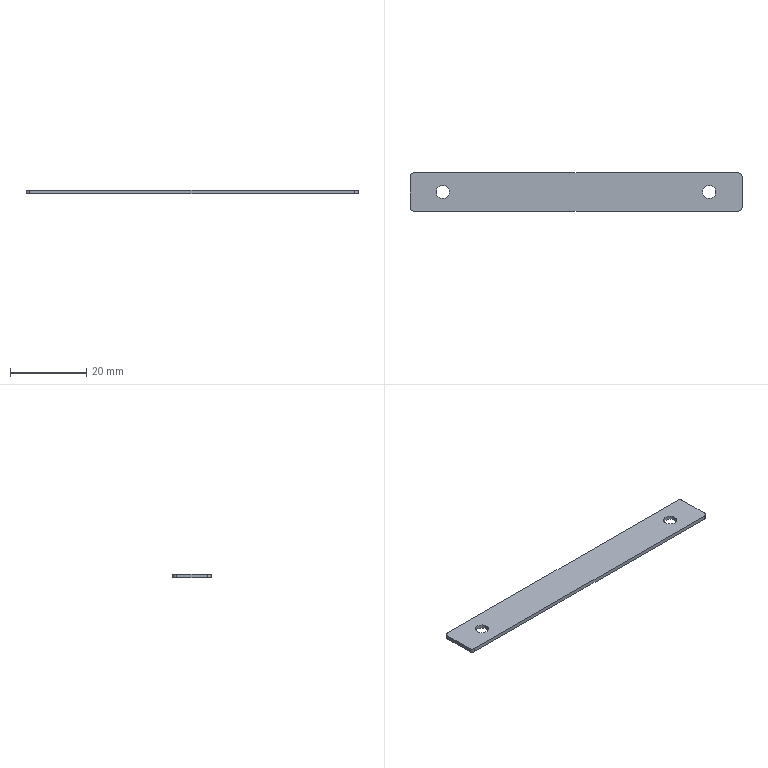Part | STEP file | LES120 steel strip pressure plate^FTH120-PD-direct-drive motor | 1 solid | 14 faces | box 87 x 10 x 1 mm | volume 849.899 mm3 | cylinder 8 | plane 6 | commonest cylinder face diameters 2 x4 3.5 x4
STEP:
#1=CARTESIAN_POINT('',(-36.65,0.,0.));
#2=VERTEX_POINT('',#1);
#3=CARTESIAN_POINT('',(-33.15,0.,0.));
#4=VERTEX_POINT('',#3);
#5=CARTESIAN_POINT('',(-34.9,0.,0.));
#6=DIRECTION('',(0.,0.,1.));
#7=DIRECTION('',(1.,0.,0.));
#8=AXIS2_PLACEMENT_3D('',#5,#6,#7);
#9=CIRCLE('',#8,1.75);
#10=EDGE_CURVE('',#2,#4,#9,.T.);
#11=ORIENTED_EDGE('',*,*,#10,.F.);
#12=CARTESIAN_POINT('',(-36.65,0.,1.));
#13=VERTEX_POINT('',#12);
#14=CARTESIAN_POINT('',(-36.65,0.,0.));
#15=DIRECTION('',(0.,0.,1.));
#16=VECTOR('',#15,1000.);
#17=LINE('',#14,#16);
#18=EDGE_CURVE('',#2,#13,#17,.T.);
#19=ORIENTED_EDGE('',*,*,#18,.T.);
#20=CARTESIAN_POINT('',(-33.15,0.,1.));
#21=VERTEX_POINT('',#20);
#22=CARTESIAN_POINT('',(-34.9,0.,1.));
#23=DIRECTION('',(0.,0.,1.));
#24=DIRECTION('',(1.,0.,0.));
#25=AXIS2_PLACEMENT_3D('',#22,#23,#24);
#26=CIRCLE('',#25,1.75);
#27=EDGE_CURVE('',#13,#21,#26,.T.);
#28=ORIENTED_EDGE('',*,*,#27,.T.);
#29=CARTESIAN_POINT('',(-33.15,0.,0.));
#30=DIRECTION('',(0.,0.,1.));
#31=VECTOR('',#30,1000.);
#32=LINE('',#29,#31);
#33=EDGE_CURVE('',#4,#21,#32,.T.);
#34=ORIENTED_EDGE('',*,*,#33,.F.);
#35=EDGE_LOOP('',(#11,#19,#28,#34));
#36=FACE_OUTER_BOUND('',#35,.T.);
#37=CARTESIAN_POINT('',(-34.9,0.,0.));
#38=DIRECTION('',(0.,0.,1.));
#39=DIRECTION('',(1.,0.,0.));
#40=AXIS2_PLACEMENT_3D('',#37,#38,#39);
#41=CYLINDRICAL_SURFACE('',#40,1.75);
#42=ADVANCED_FACE('',(#36),#41,.F.);
#43=CARTESIAN_POINT('',(33.15,0.,0.));
#44=VERTEX_POINT('',#43);
#45=CARTESIAN_POINT('',(36.65,0.,0.));
#46=VERTEX_POINT('',#45);
#47=CARTESIAN_POINT('',(34.9,0.,0.));
#48=DIRECTION('',(0.,0.,1.));
#49=DIRECTION('',(1.,0.,0.));
#50=AXIS2_PLACEMENT_3D('',#47,#48,#49);
#51=CIRCLE('',#50,1.75);
#52=EDGE_CURVE('',#44,#46,#51,.T.);
#53=ORIENTED_EDGE('',*,*,#52,.F.);
#54=CARTESIAN_POINT('',(33.15,0.,1.));
#55=VERTEX_POINT('',#54);
#56=CARTESIAN_POINT('',(33.15,0.,0.));
#57=DIRECTION('',(0.,0.,1.));
#58=VECTOR('',#57,1000.);
#59=LINE('',#56,#58);
#60=EDGE_CURVE('',#44,#55,#59,.T.);
#61=ORIENTED_EDGE('',*,*,#60,.T.);
#62=CARTESIAN_POINT('',(36.65,0.,1.));
#63=VERTEX_POINT('',#62);
#64=CARTESIAN_POINT('',(34.9,0.,1.));
#65=DIRECTION('',(0.,0.,1.));
#66=DIRECTION('',(1.,0.,0.));
#67=AXIS2_PLACEMENT_3D('',#64,#65,#66);
#68=CIRCLE('',#67,1.75);
#69=EDGE_CURVE('',#55,#63,#68,.T.);
#70=ORIENTED_EDGE('',*,*,#69,.T.);
#71=CARTESIAN_POINT('',(36.65,0.,0.));
#72=DIRECTION('',(0.,0.,1.));
#73=VECTOR('',#72,1000.);
#74=LINE('',#71,#73);
#75=EDGE_CURVE('',#46,#63,#74,.T.);
#76=ORIENTED_EDGE('',*,*,#75,.F.);
#77=EDGE_LOOP('',(#53,#61,#70,#76));
#78=FACE_OUTER_BOUND('',#77,.T.);
#79=CARTESIAN_POINT('',(34.9,0.,0.));
#80=DIRECTION('',(0.,0.,1.));
#81=DIRECTION('',(1.,0.,0.));
#82=AXIS2_PLACEMENT_3D('',#79,#80,#81);
#83=CYLINDRICAL_SURFACE('',#82,1.75);
#84=ADVANCED_FACE('',(#78),#83,.F.);
#85=CARTESIAN_POINT('',(42.5,5.,1.));
#86=VERTEX_POINT('',#85);
#87=CARTESIAN_POINT('',(43.5,4.,1.));
#88=VERTEX_POINT('',#87);
#89=CARTESIAN_POINT('',(42.5,4.,1.));
#90=DIRECTION('',(0.,0.,-1.));
#91=DIRECTION('',(-1.,0.,0.));
#92=AXIS2_PLACEMENT_3D('',#89,#90,#91);
#93=CIRCLE('',#92,1.);
#94=EDGE_CURVE('',#86,#88,#93,.T.);
#95=ORIENTED_EDGE('',*,*,#94,.F.);
#96=CARTESIAN_POINT('',(-42.5,5.,1.));
#97=VERTEX_POINT('',#96);
#98=CARTESIAN_POINT('',(0.,5.,1.));
#99=DIRECTION('',(1.,0.,0.));
#100=VECTOR('',#99,1000.);
#101=LINE('',#98,#100);
#102=EDGE_CURVE('',#97,#86,#101,.T.);
#103=ORIENTED_EDGE('',*,*,#102,.F.);
#104=CARTESIAN_POINT('',(-43.5,4.,1.));
#105=VERTEX_POINT('',#104);
#106=CARTESIAN_POINT('',(-42.5,4.,1.));
#107=DIRECTION('',(0.,0.,-1.));
#108=DIRECTION('',(-1.,0.,0.));
#109=AXIS2_PLACEMENT_3D('',#106,#107,#108);
#110=CIRCLE('',#109,1.);
#111=EDGE_CURVE('',#105,#97,#110,.T.);
#112=ORIENTED_EDGE('',*,*,#111,.F.);
#113=CARTESIAN_POINT('',(-43.5,-4.,1.));
#114=VERTEX_POINT('',#113);
#115=CARTESIAN_POINT('',(-43.5,0.,1.));
#116=DIRECTION('',(0.,1.,0.));
#117=VECTOR('',#116,1000.);
#118=LINE('',#115,#117);
#119=EDGE_CURVE('',#114,#105,#118,.T.);
#120=ORIENTED_EDGE('',*,*,#119,.F.);
#121=CARTESIAN_POINT('',(-42.5,-5.,1.));
#122=VERTEX_POINT('',#121);
#123=CARTESIAN_POINT('',(-42.5,-4.,1.));
#124=DIRECTION('',(0.,0.,-1.));
#125=DIRECTION('',(-1.,0.,0.));
#126=AXIS2_PLACEMENT_3D('',#123,#124,#125);
#127=CIRCLE('',#126,1.);
#128=EDGE_CURVE('',#122,#114,#127,.T.);
#129=ORIENTED_EDGE('',*,*,#128,.F.);
#130=CARTESIAN_POINT('',(42.5,-5.,1.));
#131=VERTEX_POINT('',#130);
#132=CARTESIAN_POINT('',(0.,-5.,1.));
#133=DIRECTION('',(-1.,0.,0.));
#134=VECTOR('',#133,1000.);
#135=LINE('',#132,#134);
#136=EDGE_CURVE('',#131,#122,#135,.T.);
#137=ORIENTED_EDGE('',*,*,#136,.F.);
#138=CARTESIAN_POINT('',(43.5,-4.,1.));
#139=VERTEX_POINT('',#138);
#140=CARTESIAN_POINT('',(42.5,-4.,1.));
#141=DIRECTION('',(0.,0.,-1.));
#142=DIRECTION('',(-1.,0.,0.));
#143=AXIS2_PLACEMENT_3D('',#140,#141,#142);
#144=CIRCLE('',#143,1.);
#145=EDGE_CURVE('',#139,#131,#144,.T.);
#146=ORIENTED_EDGE('',*,*,#145,.F.);
#147=CARTESIAN_POINT('',(43.5,0.,1.));
#148=DIRECTION('',(0.,-1.,0.));
#149=VECTOR('',#148,1000.);
#150=LINE('',#147,#149);
#151=EDGE_CURVE('',#88,#139,#150,.T.);
#152=ORIENTED_EDGE('',*,*,#151,.F.);
#153=EDGE_LOOP('',(#95,#103,#112,#120,#129,#137,#146,#152));
#154=FACE_OUTER_BOUND('',#153,.T.);
#155=CARTESIAN_POINT('',(-34.9,0.,1.));
#156=DIRECTION('',(0.,0.,1.));
#157=DIRECTION('',(1.,0.,0.));
#158=AXIS2_PLACEMENT_3D('',#155,#156,#157);
#159=CIRCLE('',#158,1.75);
#160=EDGE_CURVE('',#21,#13,#159,.T.);
#161=ORIENTED_EDGE('',*,*,#160,.F.);
#162=ORIENTED_EDGE('',*,*,#27,.F.);
#163=EDGE_LOOP('',(#161,#162));
#164=FACE_BOUND('',#163,.T.);
#165=CARTESIAN_POINT('',(34.9,0.,1.));
#166=DIRECTION('',(0.,0.,1.));
#167=DIRECTION('',(1.,0.,0.));
#168=AXIS2_PLACEMENT_3D('',#165,#166,#167);
#169=CIRCLE('',#168,1.75);
#170=EDGE_CURVE('',#63,#55,#169,.T.);
#171=ORIENTED_EDGE('',*,*,#170,.F.);
#172=ORIENTED_EDGE('',*,*,#69,.F.);
#173=EDGE_LOOP('',(#171,#172));
#174=FACE_BOUND('',#173,.T.);
#175=CARTESIAN_POINT('',(0.,0.,1.));
#176=DIRECTION('',(0.,0.,-1.));
#177=DIRECTION('',(-1.,0.,0.));
#178=AXIS2_PLACEMENT_3D('',#175,#176,#177);
#179=PLANE('',#178);
#180=ADVANCED_FACE('',(#154,#164,#174),#179,.F.);
#181=CARTESIAN_POINT('',(43.5,4.,0.));
#182=VERTEX_POINT('',#181);
#183=CARTESIAN_POINT('',(43.5,4.,1.));
#184=DIRECTION('',(0.,0.,-1.));
#185=VECTOR('',#184,1000.);
#186=LINE('',#183,#185);
#187=EDGE_CURVE('',#88,#182,#186,.T.);
#188=ORIENTED_EDGE('',*,*,#187,.F.);
#189=ORIENTED_EDGE('',*,*,#151,.T.);
#190=CARTESIAN_POINT('',(43.5,-4.,0.));
#191=VERTEX_POINT('',#190);
#192=CARTESIAN_POINT('',(43.5,-4.,1.));
#193=DIRECTION('',(0.,0.,1.));
#194=VECTOR('',#193,1000.);
#195=LINE('',#192,#194);
#196=EDGE_CURVE('',#191,#139,#195,.T.);
#197=ORIENTED_EDGE('',*,*,#196,.F.);
#198=CARTESIAN_POINT('',(43.5,-5.,0.));
#199=DIRECTION('',(0.,-1.,0.));
#200=VECTOR('',#199,1000.);
#201=LINE('',#198,#200);
#202=EDGE_CURVE('',#182,#191,#201,.T.);
#203=ORIENTED_EDGE('',*,*,#202,.F.);
#204=EDGE_LOOP('',(#188,#189,#197,#203));
#205=FACE_OUTER_BOUND('',#204,.T.);
#206=CARTESIAN_POINT('',(43.5,-5.,1.));
#207=DIRECTION('',(-1.,0.,0.));
#208=DIRECTION('',(0.,0.,1.));
#209=AXIS2_PLACEMENT_3D('',#206,#207,#208);
#210=PLANE('',#209);
#211=ADVANCED_FACE('',(#205),#210,.F.);
#212=CARTESIAN_POINT('',(42.5,5.,0.));
#213=VERTEX_POINT('',#212);
#214=CARTESIAN_POINT('',(42.5,4.,0.));
#215=DIRECTION('',(0.,0.,1.));
#216=DIRECTION('',(-1.,0.,0.));
#217=AXIS2_PLACEMENT_3D('',#214,#215,#216);
#218=CIRCLE('',#217,1.);
#219=EDGE_CURVE('',#182,#213,#218,.T.);
#220=ORIENTED_EDGE('',*,*,#219,.T.);
#221=CARTESIAN_POINT('',(42.5,5.,1.));
#222=DIRECTION('',(0.,0.,1.));
#223=VECTOR('',#222,1000.);
#224=LINE('',#221,#223);
#225=EDGE_CURVE('',#213,#86,#224,.T.);
#226=ORIENTED_EDGE('',*,*,#225,.T.);
#227=ORIENTED_EDGE('',*,*,#94,.T.);
#228=ORIENTED_EDGE('',*,*,#187,.T.);
#229=EDGE_LOOP('',(#220,#226,#227,#228));
#230=FACE_OUTER_BOUND('',#229,.T.);
#231=CARTESIAN_POINT('',(42.5,4.,1.));
#232=DIRECTION('',(0.,0.,-1.));
#233=DIRECTION('',(-1.,0.,0.));
#234=AXIS2_PLACEMENT_3D('',#231,#232,#233);
#235=CYLINDRICAL_SURFACE('',#234,1.);
#236=ADVANCED_FACE('',(#230),#235,.T.);
#237=ORIENTED_EDGE('',*,*,#225,.F.);
#238=CARTESIAN_POINT('',(-42.5,5.,0.));
#239=VERTEX_POINT('',#238);
#240=CARTESIAN_POINT('',(-43.5,5.,0.));
#241=DIRECTION('',(1.,0.,0.));
#242=VECTOR('',#241,1000.);
#243=LINE('',#240,#242);
#244=EDGE_CURVE('',#239,#213,#243,.T.);
#245=ORIENTED_EDGE('',*,*,#244,.F.);
#246=CARTESIAN_POINT('',(-42.5,5.,1.));
#247=DIRECTION('',(0.,0.,-1.));
#248=VECTOR('',#247,1000.);
#249=LINE('',#246,#248);
#250=EDGE_CURVE('',#97,#239,#249,.T.);
#251=ORIENTED_EDGE('',*,*,#250,.F.);
#252=ORIENTED_EDGE('',*,*,#102,.T.);
#253=EDGE_LOOP('',(#237,#245,#251,#252));
#254=FACE_OUTER_BOUND('',#253,.T.);
#255=CARTESIAN_POINT('',(-43.5,5.,1.));
#256=DIRECTION('',(0.,-1.,0.));
#257=DIRECTION('',(0.,0.,-1.));
#258=AXIS2_PLACEMENT_3D('',#255,#256,#257);
#259=PLANE('',#258);
#260=ADVANCED_FACE('',(#254),#259,.F.);
#261=CARTESIAN_POINT('',(-43.5,4.,0.));
#262=VERTEX_POINT('',#261);
#263=CARTESIAN_POINT('',(-42.5,4.,0.));
#264=DIRECTION('',(0.,0.,1.));
#265=DIRECTION('',(-1.,0.,0.));
#266=AXIS2_PLACEMENT_3D('',#263,#264,#265);
#267=CIRCLE('',#266,1.);
#268=EDGE_CURVE('',#239,#262,#267,.T.);
#269=ORIENTED_EDGE('',*,*,#268,.T.);
#270=CARTESIAN_POINT('',(-43.5,4.,1.));
#271=DIRECTION('',(0.,0.,1.));
#272=VECTOR('',#271,1000.);
#273=LINE('',#270,#272);
#274=EDGE_CURVE('',#262,#105,#273,.T.);
#275=ORIENTED_EDGE('',*,*,#274,.T.);
#276=ORIENTED_EDGE('',*,*,#111,.T.);
#277=ORIENTED_EDGE('',*,*,#250,.T.);
#278=EDGE_LOOP('',(#269,#275,#276,#277));
#279=FACE_OUTER_BOUND('',#278,.T.);
#280=CARTESIAN_POINT('',(-42.5,4.,1.));
#281=DIRECTION('',(0.,0.,-1.));
#282=DIRECTION('',(-1.,0.,0.));
#283=AXIS2_PLACEMENT_3D('',#280,#281,#282);
#284=CYLINDRICAL_SURFACE('',#283,1.);
#285=ADVANCED_FACE('',(#279),#284,.T.);
#286=CARTESIAN_POINT('',(-43.5,-4.,0.));
#287=VERTEX_POINT('',#286);
#288=CARTESIAN_POINT('',(-43.5,-4.,1.));
#289=DIRECTION('',(0.,0.,-1.));
#290=VECTOR('',#289,1000.);
#291=LINE('',#288,#290);
#292=EDGE_CURVE('',#114,#287,#291,.T.);
#293=ORIENTED_EDGE('',*,*,#292,.F.);
#294=ORIENTED_EDGE('',*,*,#119,.T.);
#295=ORIENTED_EDGE('',*,*,#274,.F.);
#296=CARTESIAN_POINT('',(-43.5,-5.,0.));
#297=DIRECTION('',(0.,1.,0.));
#298=VECTOR('',#297,1000.);
#299=LINE('',#296,#298);
#300=EDGE_CURVE('',#287,#262,#299,.T.);
#301=ORIENTED_EDGE('',*,*,#300,.F.);
#302=EDGE_LOOP('',(#293,#294,#295,#301));
#303=FACE_OUTER_BOUND('',#302,.T.);
#304=CARTESIAN_POINT('',(-43.5,-5.,1.));
#305=DIRECTION('',(1.,0.,0.));
#306=DIRECTION('',(0.,0.,-1.));
#307=AXIS2_PLACEMENT_3D('',#304,#305,#306);
#308=PLANE('',#307);
#309=ADVANCED_FACE('',(#303),#308,.F.);
#310=CARTESIAN_POINT('',(-42.5,-5.,0.));
#311=VERTEX_POINT('',#310);
#312=CARTESIAN_POINT('',(-42.5,-4.,0.));
#313=DIRECTION('',(0.,0.,1.));
#314=DIRECTION('',(-1.,0.,0.));
#315=AXIS2_PLACEMENT_3D('',#312,#313,#314);
#316=CIRCLE('',#315,1.);
#317=EDGE_CURVE('',#287,#311,#316,.T.);
#318=ORIENTED_EDGE('',*,*,#317,.T.);
#319=CARTESIAN_POINT('',(-42.5,-5.,1.));
#320=DIRECTION('',(0.,0.,1.));
#321=VECTOR('',#320,1000.);
#322=LINE('',#319,#321);
#323=EDGE_CURVE('',#311,#122,#322,.T.);
#324=ORIENTED_EDGE('',*,*,#323,.T.);
#325=ORIENTED_EDGE('',*,*,#128,.T.);
#326=ORIENTED_EDGE('',*,*,#292,.T.);
#327=EDGE_LOOP('',(#318,#324,#325,#326));
#328=FACE_OUTER_BOUND('',#327,.T.);
#329=CARTESIAN_POINT('',(-42.5,-4.,1.));
#330=DIRECTION('',(0.,0.,-1.));
#331=DIRECTION('',(-1.,0.,0.));
#332=AXIS2_PLACEMENT_3D('',#329,#330,#331);
#333=CYLINDRICAL_SURFACE('',#332,1.);
#334=ADVANCED_FACE('',(#328),#333,.T.);
#335=CARTESIAN_POINT('',(42.5,-5.,0.));
#336=VERTEX_POINT('',#335);
#337=CARTESIAN_POINT('',(42.5,-5.,1.));
#338=DIRECTION('',(0.,0.,-1.));
#339=VECTOR('',#338,1000.);
#340=LINE('',#337,#339);
#341=EDGE_CURVE('',#131,#336,#340,.T.);
#342=ORIENTED_EDGE('',*,*,#341,.F.);
#343=ORIENTED_EDGE('',*,*,#136,.T.);
#344=ORIENTED_EDGE('',*,*,#323,.F.);
#345=CARTESIAN_POINT('',(-43.5,-5.,0.));
#346=DIRECTION('',(-1.,0.,0.));
#347=VECTOR('',#346,1000.);
#348=LINE('',#345,#347);
#349=EDGE_CURVE('',#336,#311,#348,.T.);
#350=ORIENTED_EDGE('',*,*,#349,.F.);
#351=EDGE_LOOP('',(#342,#343,#344,#350));
#352=FACE_OUTER_BOUND('',#351,.T.);
#353=CARTESIAN_POINT('',(-43.5,-5.,1.));
#354=DIRECTION('',(0.,1.,0.));
#355=DIRECTION('',(0.,0.,1.));
#356=AXIS2_PLACEMENT_3D('',#353,#354,#355);
#357=PLANE('',#356);
#358=ADVANCED_FACE('',(#352),#357,.F.);
#359=CARTESIAN_POINT('',(42.5,-4.,0.));
#360=DIRECTION('',(0.,0.,1.));
#361=DIRECTION('',(-1.,0.,0.));
#362=AXIS2_PLACEMENT_3D('',#359,#360,#361);
#363=CIRCLE('',#362,1.);
#364=EDGE_CURVE('',#336,#191,#363,.T.);
#365=ORIENTED_EDGE('',*,*,#364,.T.);
#366=ORIENTED_EDGE('',*,*,#196,.T.);
#367=ORIENTED_EDGE('',*,*,#145,.T.);
#368=ORIENTED_EDGE('',*,*,#341,.T.);
#369=EDGE_LOOP('',(#365,#366,#367,#368));
#370=FACE_OUTER_BOUND('',#369,.T.);
#371=CARTESIAN_POINT('',(42.5,-4.,1.));
#372=DIRECTION('',(0.,0.,-1.));
#373=DIRECTION('',(-1.,0.,0.));
#374=AXIS2_PLACEMENT_3D('',#371,#372,#373);
#375=CYLINDRICAL_SURFACE('',#374,1.);
#376=ADVANCED_FACE('',(#370),#375,.T.);
#377=ORIENTED_EDGE('',*,*,#18,.F.);
#378=CARTESIAN_POINT('',(-34.9,0.,0.));
#379=DIRECTION('',(0.,0.,1.));
#380=DIRECTION('',(1.,0.,0.));
#381=AXIS2_PLACEMENT_3D('',#378,#379,#380);
#382=CIRCLE('',#381,1.75);
#383=EDGE_CURVE('',#4,#2,#382,.T.);
#384=ORIENTED_EDGE('',*,*,#383,.F.);
#385=ORIENTED_EDGE('',*,*,#33,.T.);
#386=ORIENTED_EDGE('',*,*,#160,.T.);
#387=EDGE_LOOP('',(#377,#384,#385,#386));
#388=FACE_OUTER_BOUND('',#387,.T.);
#389=CARTESIAN_POINT('',(-34.9,0.,0.));
#390=DIRECTION('',(0.,0.,1.));
#391=DIRECTION('',(1.,0.,0.));
#392=AXIS2_PLACEMENT_3D('',#389,#390,#391);
#393=CYLINDRICAL_SURFACE('',#392,1.75);
#394=ADVANCED_FACE('',(#388),#393,.F.);
#395=ORIENTED_EDGE('',*,*,#60,.F.);
#396=CARTESIAN_POINT('',(34.9,0.,0.));
#397=DIRECTION('',(0.,0.,1.));
#398=DIRECTION('',(1.,0.,0.));
#399=AXIS2_PLACEMENT_3D('',#396,#397,#398);
#400=CIRCLE('',#399,1.75);
#401=EDGE_CURVE('',#46,#44,#400,.T.);
#402=ORIENTED_EDGE('',*,*,#401,.F.);
#403=ORIENTED_EDGE('',*,*,#75,.T.);
#404=ORIENTED_EDGE('',*,*,#170,.T.);
#405=EDGE_LOOP('',(#395,#402,#403,#404));
#406=FACE_OUTER_BOUND('',#405,.T.);
#407=CARTESIAN_POINT('',(34.9,0.,0.));
#408=DIRECTION('',(0.,0.,1.));
#409=DIRECTION('',(1.,0.,0.));
#410=AXIS2_PLACEMENT_3D('',#407,#408,#409);
#411=CYLINDRICAL_SURFACE('',#410,1.75);
#412=ADVANCED_FACE('',(#406),#411,.F.);
#413=ORIENTED_EDGE('',*,*,#300,.T.);
#414=ORIENTED_EDGE('',*,*,#268,.F.);
#415=ORIENTED_EDGE('',*,*,#244,.T.);
#416=ORIENTED_EDGE('',*,*,#219,.F.);
#417=ORIENTED_EDGE('',*,*,#202,.T.);
#418=ORIENTED_EDGE('',*,*,#364,.F.);
#419=ORIENTED_EDGE('',*,*,#349,.T.);
#420=ORIENTED_EDGE('',*,*,#317,.F.);
#421=EDGE_LOOP('',(#413,#414,#415,#416,#417,#418,#419,#420));
#422=FACE_OUTER_BOUND('',#421,.T.);
#423=ORIENTED_EDGE('',*,*,#383,.T.);
#424=ORIENTED_EDGE('',*,*,#10,.T.);
#425=EDGE_LOOP('',(#423,#424));
#426=FACE_BOUND('',#425,.T.);
#427=ORIENTED_EDGE('',*,*,#401,.T.);
#428=ORIENTED_EDGE('',*,*,#52,.T.);
#429=EDGE_LOOP('',(#427,#428));
#430=FACE_BOUND('',#429,.T.);
#431=CARTESIAN_POINT('',(0.,0.,0.));
#432=DIRECTION('',(0.,0.,-1.));
#433=DIRECTION('',(-1.,0.,0.));
#434=AXIS2_PLACEMENT_3D('',#431,#432,#433);
#435=PLANE('',#434);
#436=ADVANCED_FACE('',(#422,#426,#430),#435,.T.);
#437=CLOSED_SHELL('',(#42,#84,#180,#211,#236,#260,#285,#309,#334,#358,#376,#394,#412,#436));
#438=MANIFOLD_SOLID_BREP('',#437);
#439=CARTESIAN_POINT('',(0.,0.,0.));
#440=DIRECTION('',(0.,0.,1.));
#441=DIRECTION('',(1.,0.,0.));
#442=AXIS2_PLACEMENT_3D('',#439,#440,#441);
#443=(LENGTH_UNIT()NAMED_UNIT(*)SI_UNIT(.MILLI.,.METRE.));
#444=UNCERTAINTY_MEASURE_WITH_UNIT(LENGTH_MEASURE(0.00001),#443,'','');
#445=(NAMED_UNIT(*)PLANE_ANGLE_UNIT()SI_UNIT($,.RADIAN.));
#446=(NAMED_UNIT(*)SI_UNIT($,.STERADIAN.)SOLID_ANGLE_UNIT());
#447=(GEOMETRIC_REPRESENTATION_CONTEXT(3)GLOBAL_UNCERTAINTY_ASSIGNED_CONTEXT((#444))GLOBAL_UNIT_ASSIGNED_CONTEXT((#443,#445,#446))REPRESENTATION_CONTEXT('',''));
#448=ADVANCED_BREP_SHAPE_REPRESENTATION('',(#438,#442),#447);